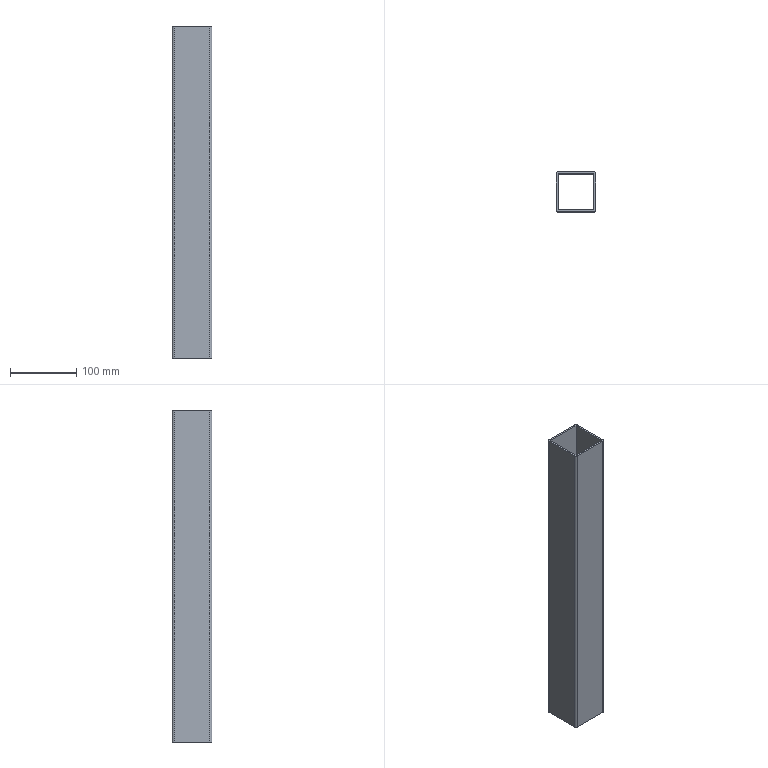Part | STEP file | X77-03111 | 1 solid | 14 faces | box 60 x 60 x 500 mm | volume 338137 mm3 | plane 10 | cylinder 4 | commonest cylinder face diameters 6 x4
STEP:
#1=CARTESIAN_POINT('',(0.,3.,500.));
#2=VERTEX_POINT('',#1);
#3=CARTESIAN_POINT('',(3.,0.,500.));
#4=VERTEX_POINT('',#3);
#5=CARTESIAN_POINT('',(3.,3.,500.));
#6=DIRECTION('',(0.,0.,1.));
#7=DIRECTION('',(1.,0.,0.));
#8=AXIS2_PLACEMENT_3D('',#5,#6,#7);
#9=CIRCLE('',#8,3.);
#10=EDGE_CURVE('',#2,#4,#9,.T.);
#11=ORIENTED_EDGE('',*,*,#10,.T.);
#12=CARTESIAN_POINT('',(57.,0.,500.));
#13=VERTEX_POINT('',#12);
#14=CARTESIAN_POINT('',(3.,0.,500.));
#15=DIRECTION('',(1.,0.,0.));
#16=VECTOR('',#15,1000.);
#17=LINE('',#14,#16);
#18=EDGE_CURVE('',#4,#13,#17,.T.);
#19=ORIENTED_EDGE('',*,*,#18,.T.);
#20=CARTESIAN_POINT('',(60.,3.,500.));
#21=VERTEX_POINT('',#20);
#22=CARTESIAN_POINT('',(57.,3.,500.));
#23=DIRECTION('',(0.,0.,1.));
#24=DIRECTION('',(1.,0.,0.));
#25=AXIS2_PLACEMENT_3D('',#22,#23,#24);
#26=CIRCLE('',#25,3.);
#27=EDGE_CURVE('',#13,#21,#26,.T.);
#28=ORIENTED_EDGE('',*,*,#27,.T.);
#29=CARTESIAN_POINT('',(60.,57.,500.));
#30=VERTEX_POINT('',#29);
#31=CARTESIAN_POINT('',(60.,3.,500.));
#32=DIRECTION('',(0.,1.,0.));
#33=VECTOR('',#32,1000.);
#34=LINE('',#31,#33);
#35=EDGE_CURVE('',#21,#30,#34,.T.);
#36=ORIENTED_EDGE('',*,*,#35,.T.);
#37=CARTESIAN_POINT('',(57.,60.,500.));
#38=VERTEX_POINT('',#37);
#39=CARTESIAN_POINT('',(57.,57.,500.));
#40=DIRECTION('',(0.,0.,1.));
#41=DIRECTION('',(1.,0.,0.));
#42=AXIS2_PLACEMENT_3D('',#39,#40,#41);
#43=CIRCLE('',#42,3.);
#44=EDGE_CURVE('',#30,#38,#43,.T.);
#45=ORIENTED_EDGE('',*,*,#44,.T.);
#46=CARTESIAN_POINT('',(3.,60.,500.));
#47=VERTEX_POINT('',#46);
#48=CARTESIAN_POINT('',(3.,60.,500.));
#49=DIRECTION('',(-1.,0.,0.));
#50=VECTOR('',#49,1000.);
#51=LINE('',#48,#50);
#52=EDGE_CURVE('',#38,#47,#51,.T.);
#53=ORIENTED_EDGE('',*,*,#52,.T.);
#54=CARTESIAN_POINT('',(0.,57.,500.));
#55=VERTEX_POINT('',#54);
#56=CARTESIAN_POINT('',(3.,57.,500.));
#57=DIRECTION('',(0.,0.,1.));
#58=DIRECTION('',(1.,0.,0.));
#59=AXIS2_PLACEMENT_3D('',#56,#57,#58);
#60=CIRCLE('',#59,3.);
#61=EDGE_CURVE('',#47,#55,#60,.T.);
#62=ORIENTED_EDGE('',*,*,#61,.T.);
#63=CARTESIAN_POINT('',(0.,3.,500.));
#64=DIRECTION('',(0.,-1.,0.));
#65=VECTOR('',#64,1000.);
#66=LINE('',#63,#65);
#67=EDGE_CURVE('',#55,#2,#66,.T.);
#68=ORIENTED_EDGE('',*,*,#67,.T.);
#69=EDGE_LOOP('',(#11,#19,#28,#36,#45,#53,#62,#68));
#70=FACE_OUTER_BOUND('',#69,.T.);
#71=CARTESIAN_POINT('',(3.,3.,500.));
#72=VERTEX_POINT('',#71);
#73=CARTESIAN_POINT('',(57.,3.,500.));
#74=VERTEX_POINT('',#73);
#75=CARTESIAN_POINT('',(3.,3.,500.));
#76=DIRECTION('',(1.,0.,0.));
#77=VECTOR('',#76,1000.);
#78=LINE('',#75,#77);
#79=EDGE_CURVE('',#72,#74,#78,.T.);
#80=ORIENTED_EDGE('',*,*,#79,.F.);
#81=CARTESIAN_POINT('',(3.,57.,500.));
#82=VERTEX_POINT('',#81);
#83=CARTESIAN_POINT('',(3.,3.,500.));
#84=DIRECTION('',(0.,-1.,0.));
#85=VECTOR('',#84,1000.);
#86=LINE('',#83,#85);
#87=EDGE_CURVE('',#82,#72,#86,.T.);
#88=ORIENTED_EDGE('',*,*,#87,.F.);
#89=CARTESIAN_POINT('',(57.,57.,500.));
#90=VERTEX_POINT('',#89);
#91=CARTESIAN_POINT('',(3.,57.,500.));
#92=DIRECTION('',(-1.,0.,0.));
#93=VECTOR('',#92,1000.);
#94=LINE('',#91,#93);
#95=EDGE_CURVE('',#90,#82,#94,.T.);
#96=ORIENTED_EDGE('',*,*,#95,.F.);
#97=CARTESIAN_POINT('',(57.,3.,500.));
#98=DIRECTION('',(0.,1.,0.));
#99=VECTOR('',#98,1000.);
#100=LINE('',#97,#99);
#101=EDGE_CURVE('',#74,#90,#100,.T.);
#102=ORIENTED_EDGE('',*,*,#101,.F.);
#103=EDGE_LOOP('',(#80,#88,#96,#102));
#104=FACE_BOUND('',#103,.T.);
#105=CARTESIAN_POINT('',(3.,3.,500.));
#106=DIRECTION('',(0.,0.,1.));
#107=DIRECTION('',(1.,0.,0.));
#108=AXIS2_PLACEMENT_3D('',#105,#106,#107);
#109=PLANE('',#108);
#110=ADVANCED_FACE('',(#70,#104),#109,.T.);
#111=CARTESIAN_POINT('',(0.,3.,0.));
#112=VERTEX_POINT('',#111);
#113=CARTESIAN_POINT('',(3.,0.,0.));
#114=VERTEX_POINT('',#113);
#115=CARTESIAN_POINT('',(3.,3.,0.));
#116=DIRECTION('',(0.,0.,1.));
#117=DIRECTION('',(1.,0.,0.));
#118=AXIS2_PLACEMENT_3D('',#115,#116,#117);
#119=CIRCLE('',#118,3.);
#120=EDGE_CURVE('',#112,#114,#119,.T.);
#121=ORIENTED_EDGE('',*,*,#120,.F.);
#122=CARTESIAN_POINT('',(0.,57.,0.));
#123=VERTEX_POINT('',#122);
#124=CARTESIAN_POINT('',(0.,3.,0.));
#125=DIRECTION('',(0.,-1.,0.));
#126=VECTOR('',#125,1000.);
#127=LINE('',#124,#126);
#128=EDGE_CURVE('',#123,#112,#127,.T.);
#129=ORIENTED_EDGE('',*,*,#128,.F.);
#130=CARTESIAN_POINT('',(3.,60.,0.));
#131=VERTEX_POINT('',#130);
#132=CARTESIAN_POINT('',(3.,57.,0.));
#133=DIRECTION('',(0.,0.,1.));
#134=DIRECTION('',(1.,0.,0.));
#135=AXIS2_PLACEMENT_3D('',#132,#133,#134);
#136=CIRCLE('',#135,3.);
#137=EDGE_CURVE('',#131,#123,#136,.T.);
#138=ORIENTED_EDGE('',*,*,#137,.F.);
#139=CARTESIAN_POINT('',(57.,60.,0.));
#140=VERTEX_POINT('',#139);
#141=CARTESIAN_POINT('',(3.,60.,0.));
#142=DIRECTION('',(-1.,0.,0.));
#143=VECTOR('',#142,1000.);
#144=LINE('',#141,#143);
#145=EDGE_CURVE('',#140,#131,#144,.T.);
#146=ORIENTED_EDGE('',*,*,#145,.F.);
#147=CARTESIAN_POINT('',(60.,57.,0.));
#148=VERTEX_POINT('',#147);
#149=CARTESIAN_POINT('',(57.,57.,0.));
#150=DIRECTION('',(0.,0.,1.));
#151=DIRECTION('',(1.,0.,0.));
#152=AXIS2_PLACEMENT_3D('',#149,#150,#151);
#153=CIRCLE('',#152,3.);
#154=EDGE_CURVE('',#148,#140,#153,.T.);
#155=ORIENTED_EDGE('',*,*,#154,.F.);
#156=CARTESIAN_POINT('',(60.,3.,0.));
#157=VERTEX_POINT('',#156);
#158=CARTESIAN_POINT('',(60.,3.,0.));
#159=DIRECTION('',(0.,1.,0.));
#160=VECTOR('',#159,1000.);
#161=LINE('',#158,#160);
#162=EDGE_CURVE('',#157,#148,#161,.T.);
#163=ORIENTED_EDGE('',*,*,#162,.F.);
#164=CARTESIAN_POINT('',(57.,0.,0.));
#165=VERTEX_POINT('',#164);
#166=CARTESIAN_POINT('',(57.,3.,0.));
#167=DIRECTION('',(0.,0.,1.));
#168=DIRECTION('',(1.,0.,0.));
#169=AXIS2_PLACEMENT_3D('',#166,#167,#168);
#170=CIRCLE('',#169,3.);
#171=EDGE_CURVE('',#165,#157,#170,.T.);
#172=ORIENTED_EDGE('',*,*,#171,.F.);
#173=CARTESIAN_POINT('',(3.,0.,0.));
#174=DIRECTION('',(1.,0.,0.));
#175=VECTOR('',#174,1000.);
#176=LINE('',#173,#175);
#177=EDGE_CURVE('',#114,#165,#176,.T.);
#178=ORIENTED_EDGE('',*,*,#177,.F.);
#179=EDGE_LOOP('',(#121,#129,#138,#146,#155,#163,#172,#178));
#180=FACE_OUTER_BOUND('',#179,.T.);
#181=CARTESIAN_POINT('',(3.,57.,0.));
#182=VERTEX_POINT('',#181);
#183=CARTESIAN_POINT('',(3.,3.,0.));
#184=VERTEX_POINT('',#183);
#185=CARTESIAN_POINT('',(3.,3.,0.));
#186=DIRECTION('',(0.,-1.,0.));
#187=VECTOR('',#186,1000.);
#188=LINE('',#185,#187);
#189=EDGE_CURVE('',#182,#184,#188,.T.);
#190=ORIENTED_EDGE('',*,*,#189,.T.);
#191=CARTESIAN_POINT('',(57.,3.,0.));
#192=VERTEX_POINT('',#191);
#193=CARTESIAN_POINT('',(3.,3.,0.));
#194=DIRECTION('',(1.,0.,0.));
#195=VECTOR('',#194,1000.);
#196=LINE('',#193,#195);
#197=EDGE_CURVE('',#184,#192,#196,.T.);
#198=ORIENTED_EDGE('',*,*,#197,.T.);
#199=CARTESIAN_POINT('',(57.,57.,0.));
#200=VERTEX_POINT('',#199);
#201=CARTESIAN_POINT('',(57.,3.,0.));
#202=DIRECTION('',(0.,1.,0.));
#203=VECTOR('',#202,1000.);
#204=LINE('',#201,#203);
#205=EDGE_CURVE('',#192,#200,#204,.T.);
#206=ORIENTED_EDGE('',*,*,#205,.T.);
#207=CARTESIAN_POINT('',(3.,57.,0.));
#208=DIRECTION('',(-1.,0.,0.));
#209=VECTOR('',#208,1000.);
#210=LINE('',#207,#209);
#211=EDGE_CURVE('',#200,#182,#210,.T.);
#212=ORIENTED_EDGE('',*,*,#211,.T.);
#213=EDGE_LOOP('',(#190,#198,#206,#212));
#214=FACE_BOUND('',#213,.T.);
#215=CARTESIAN_POINT('',(3.,3.,0.));
#216=DIRECTION('',(0.,0.,1.));
#217=DIRECTION('',(1.,0.,0.));
#218=AXIS2_PLACEMENT_3D('',#215,#216,#217);
#219=PLANE('',#218);
#220=ADVANCED_FACE('',(#180,#214),#219,.F.);
#221=ORIENTED_EDGE('',*,*,#120,.T.);
#222=CARTESIAN_POINT('',(3.,0.,500.));
#223=DIRECTION('',(0.,0.,-1.));
#224=VECTOR('',#223,1000.);
#225=LINE('',#222,#224);
#226=EDGE_CURVE('',#4,#114,#225,.T.);
#227=ORIENTED_EDGE('',*,*,#226,.F.);
#228=ORIENTED_EDGE('',*,*,#10,.F.);
#229=CARTESIAN_POINT('',(0.,3.,500.));
#230=DIRECTION('',(0.,0.,-1.));
#231=VECTOR('',#230,1000.);
#232=LINE('',#229,#231);
#233=EDGE_CURVE('',#2,#112,#232,.T.);
#234=ORIENTED_EDGE('',*,*,#233,.T.);
#235=EDGE_LOOP('',(#221,#227,#228,#234));
#236=FACE_OUTER_BOUND('',#235,.T.);
#237=CARTESIAN_POINT('',(3.,3.,500.));
#238=DIRECTION('',(0.,0.,-1.));
#239=DIRECTION('',(-1.,0.,0.));
#240=AXIS2_PLACEMENT_3D('',#237,#238,#239);
#241=CYLINDRICAL_SURFACE('',#240,3.);
#242=ADVANCED_FACE('',(#236),#241,.T.);
#243=ORIENTED_EDGE('',*,*,#177,.T.);
#244=CARTESIAN_POINT('',(57.,0.,500.));
#245=DIRECTION('',(0.,0.,-1.));
#246=VECTOR('',#245,1000.);
#247=LINE('',#244,#246);
#248=EDGE_CURVE('',#13,#165,#247,.T.);
#249=ORIENTED_EDGE('',*,*,#248,.F.);
#250=ORIENTED_EDGE('',*,*,#18,.F.);
#251=ORIENTED_EDGE('',*,*,#226,.T.);
#252=EDGE_LOOP('',(#243,#249,#250,#251));
#253=FACE_OUTER_BOUND('',#252,.T.);
#254=CARTESIAN_POINT('',(3.,0.,500.));
#255=DIRECTION('',(0.,1.,0.));
#256=DIRECTION('',(0.,0.,1.));
#257=AXIS2_PLACEMENT_3D('',#254,#255,#256);
#258=PLANE('',#257);
#259=ADVANCED_FACE('',(#253),#258,.F.);
#260=ORIENTED_EDGE('',*,*,#171,.T.);
#261=CARTESIAN_POINT('',(60.,3.,500.));
#262=DIRECTION('',(0.,0.,-1.));
#263=VECTOR('',#262,1000.);
#264=LINE('',#261,#263);
#265=EDGE_CURVE('',#21,#157,#264,.T.);
#266=ORIENTED_EDGE('',*,*,#265,.F.);
#267=ORIENTED_EDGE('',*,*,#27,.F.);
#268=ORIENTED_EDGE('',*,*,#248,.T.);
#269=EDGE_LOOP('',(#260,#266,#267,#268));
#270=FACE_OUTER_BOUND('',#269,.T.);
#271=CARTESIAN_POINT('',(57.,3.,500.));
#272=DIRECTION('',(0.,0.,-1.));
#273=DIRECTION('',(-1.,0.,0.));
#274=AXIS2_PLACEMENT_3D('',#271,#272,#273);
#275=CYLINDRICAL_SURFACE('',#274,3.);
#276=ADVANCED_FACE('',(#270),#275,.T.);
#277=ORIENTED_EDGE('',*,*,#162,.T.);
#278=CARTESIAN_POINT('',(60.,57.,500.));
#279=DIRECTION('',(0.,0.,-1.));
#280=VECTOR('',#279,1000.);
#281=LINE('',#278,#280);
#282=EDGE_CURVE('',#30,#148,#281,.T.);
#283=ORIENTED_EDGE('',*,*,#282,.F.);
#284=ORIENTED_EDGE('',*,*,#35,.F.);
#285=ORIENTED_EDGE('',*,*,#265,.T.);
#286=EDGE_LOOP('',(#277,#283,#284,#285));
#287=FACE_OUTER_BOUND('',#286,.T.);
#288=CARTESIAN_POINT('',(60.,3.,500.));
#289=DIRECTION('',(-1.,0.,0.));
#290=DIRECTION('',(0.,0.,1.));
#291=AXIS2_PLACEMENT_3D('',#288,#289,#290);
#292=PLANE('',#291);
#293=ADVANCED_FACE('',(#287),#292,.F.);
#294=ORIENTED_EDGE('',*,*,#154,.T.);
#295=CARTESIAN_POINT('',(57.,60.,500.));
#296=DIRECTION('',(0.,0.,-1.));
#297=VECTOR('',#296,1000.);
#298=LINE('',#295,#297);
#299=EDGE_CURVE('',#38,#140,#298,.T.);
#300=ORIENTED_EDGE('',*,*,#299,.F.);
#301=ORIENTED_EDGE('',*,*,#44,.F.);
#302=ORIENTED_EDGE('',*,*,#282,.T.);
#303=EDGE_LOOP('',(#294,#300,#301,#302));
#304=FACE_OUTER_BOUND('',#303,.T.);
#305=CARTESIAN_POINT('',(57.,57.,500.));
#306=DIRECTION('',(0.,0.,-1.));
#307=DIRECTION('',(-1.,0.,0.));
#308=AXIS2_PLACEMENT_3D('',#305,#306,#307);
#309=CYLINDRICAL_SURFACE('',#308,3.);
#310=ADVANCED_FACE('',(#304),#309,.T.);
#311=ORIENTED_EDGE('',*,*,#145,.T.);
#312=CARTESIAN_POINT('',(3.,60.,500.));
#313=DIRECTION('',(0.,0.,-1.));
#314=VECTOR('',#313,1000.);
#315=LINE('',#312,#314);
#316=EDGE_CURVE('',#47,#131,#315,.T.);
#317=ORIENTED_EDGE('',*,*,#316,.F.);
#318=ORIENTED_EDGE('',*,*,#52,.F.);
#319=ORIENTED_EDGE('',*,*,#299,.T.);
#320=EDGE_LOOP('',(#311,#317,#318,#319));
#321=FACE_OUTER_BOUND('',#320,.T.);
#322=CARTESIAN_POINT('',(3.,60.,500.));
#323=DIRECTION('',(0.,-1.,0.));
#324=DIRECTION('',(0.,0.,-1.));
#325=AXIS2_PLACEMENT_3D('',#322,#323,#324);
#326=PLANE('',#325);
#327=ADVANCED_FACE('',(#321),#326,.F.);
#328=ORIENTED_EDGE('',*,*,#137,.T.);
#329=CARTESIAN_POINT('',(0.,57.,500.));
#330=DIRECTION('',(0.,0.,-1.));
#331=VECTOR('',#330,1000.);
#332=LINE('',#329,#331);
#333=EDGE_CURVE('',#55,#123,#332,.T.);
#334=ORIENTED_EDGE('',*,*,#333,.F.);
#335=ORIENTED_EDGE('',*,*,#61,.F.);
#336=ORIENTED_EDGE('',*,*,#316,.T.);
#337=EDGE_LOOP('',(#328,#334,#335,#336));
#338=FACE_OUTER_BOUND('',#337,.T.);
#339=CARTESIAN_POINT('',(3.,57.,500.));
#340=DIRECTION('',(0.,0.,-1.));
#341=DIRECTION('',(-1.,0.,0.));
#342=AXIS2_PLACEMENT_3D('',#339,#340,#341);
#343=CYLINDRICAL_SURFACE('',#342,3.);
#344=ADVANCED_FACE('',(#338),#343,.T.);
#345=ORIENTED_EDGE('',*,*,#128,.T.);
#346=ORIENTED_EDGE('',*,*,#233,.F.);
#347=ORIENTED_EDGE('',*,*,#67,.F.);
#348=ORIENTED_EDGE('',*,*,#333,.T.);
#349=EDGE_LOOP('',(#345,#346,#347,#348));
#350=FACE_OUTER_BOUND('',#349,.T.);
#351=CARTESIAN_POINT('',(0.,3.,500.));
#352=DIRECTION('',(1.,0.,0.));
#353=DIRECTION('',(0.,0.,-1.));
#354=AXIS2_PLACEMENT_3D('',#351,#352,#353);
#355=PLANE('',#354);
#356=ADVANCED_FACE('',(#350),#355,.F.);
#357=ORIENTED_EDGE('',*,*,#189,.F.);
#358=CARTESIAN_POINT('',(3.,57.,500.));
#359=DIRECTION('',(0.,0.,-1.));
#360=VECTOR('',#359,1000.);
#361=LINE('',#358,#360);
#362=EDGE_CURVE('',#82,#182,#361,.T.);
#363=ORIENTED_EDGE('',*,*,#362,.F.);
#364=ORIENTED_EDGE('',*,*,#87,.T.);
#365=CARTESIAN_POINT('',(3.,3.,500.));
#366=DIRECTION('',(0.,0.,-1.));
#367=VECTOR('',#366,1000.);
#368=LINE('',#365,#367);
#369=EDGE_CURVE('',#72,#184,#368,.T.);
#370=ORIENTED_EDGE('',*,*,#369,.T.);
#371=EDGE_LOOP('',(#357,#363,#364,#370));
#372=FACE_OUTER_BOUND('',#371,.T.);
#373=CARTESIAN_POINT('',(3.,3.,500.));
#374=DIRECTION('',(1.,0.,0.));
#375=DIRECTION('',(0.,0.,-1.));
#376=AXIS2_PLACEMENT_3D('',#373,#374,#375);
#377=PLANE('',#376);
#378=ADVANCED_FACE('',(#372),#377,.T.);
#379=ORIENTED_EDGE('',*,*,#197,.F.);
#380=ORIENTED_EDGE('',*,*,#369,.F.);
#381=ORIENTED_EDGE('',*,*,#79,.T.);
#382=CARTESIAN_POINT('',(57.,3.,500.));
#383=DIRECTION('',(0.,0.,-1.));
#384=VECTOR('',#383,1000.);
#385=LINE('',#382,#384);
#386=EDGE_CURVE('',#74,#192,#385,.T.);
#387=ORIENTED_EDGE('',*,*,#386,.T.);
#388=EDGE_LOOP('',(#379,#380,#381,#387));
#389=FACE_OUTER_BOUND('',#388,.T.);
#390=CARTESIAN_POINT('',(3.,3.,500.));
#391=DIRECTION('',(0.,1.,0.));
#392=DIRECTION('',(0.,0.,1.));
#393=AXIS2_PLACEMENT_3D('',#390,#391,#392);
#394=PLANE('',#393);
#395=ADVANCED_FACE('',(#389),#394,.T.);
#396=ORIENTED_EDGE('',*,*,#205,.F.);
#397=ORIENTED_EDGE('',*,*,#386,.F.);
#398=ORIENTED_EDGE('',*,*,#101,.T.);
#399=CARTESIAN_POINT('',(57.,57.,500.));
#400=DIRECTION('',(0.,0.,-1.));
#401=VECTOR('',#400,1000.);
#402=LINE('',#399,#401);
#403=EDGE_CURVE('',#90,#200,#402,.T.);
#404=ORIENTED_EDGE('',*,*,#403,.T.);
#405=EDGE_LOOP('',(#396,#397,#398,#404));
#406=FACE_OUTER_BOUND('',#405,.T.);
#407=CARTESIAN_POINT('',(57.,3.,500.));
#408=DIRECTION('',(-1.,0.,0.));
#409=DIRECTION('',(0.,0.,1.));
#410=AXIS2_PLACEMENT_3D('',#407,#408,#409);
#411=PLANE('',#410);
#412=ADVANCED_FACE('',(#406),#411,.T.);
#413=ORIENTED_EDGE('',*,*,#211,.F.);
#414=ORIENTED_EDGE('',*,*,#403,.F.);
#415=ORIENTED_EDGE('',*,*,#95,.T.);
#416=ORIENTED_EDGE('',*,*,#362,.T.);
#417=EDGE_LOOP('',(#413,#414,#415,#416));
#418=FACE_OUTER_BOUND('',#417,.T.);
#419=CARTESIAN_POINT('',(3.,57.,500.));
#420=DIRECTION('',(0.,-1.,0.));
#421=DIRECTION('',(0.,0.,-1.));
#422=AXIS2_PLACEMENT_3D('',#419,#420,#421);
#423=PLANE('',#422);
#424=ADVANCED_FACE('',(#418),#423,.T.);
#425=CLOSED_SHELL('',(#110,#220,#242,#259,#276,#293,#310,#327,#344,#356,#378,#395,#412,#424));
#426=MANIFOLD_SOLID_BREP('',#425);
#427=CARTESIAN_POINT('',(0.,0.,0.));
#428=DIRECTION('',(0.,0.,1.));
#429=DIRECTION('',(1.,0.,0.));
#430=AXIS2_PLACEMENT_3D('',#427,#428,#429);
#431=(LENGTH_UNIT()NAMED_UNIT(*)SI_UNIT(.MILLI.,.METRE.));
#432=UNCERTAINTY_MEASURE_WITH_UNIT(LENGTH_MEASURE(0.00001),#431,'','');
#433=(NAMED_UNIT(*)PLANE_ANGLE_UNIT()SI_UNIT($,.RADIAN.));
#434=(NAMED_UNIT(*)SI_UNIT($,.STERADIAN.)SOLID_ANGLE_UNIT());
#435=(GEOMETRIC_REPRESENTATION_CONTEXT(3)GLOBAL_UNCERTAINTY_ASSIGNED_CONTEXT((#432))GLOBAL_UNIT_ASSIGNED_CONTEXT((#431,#433,#434))REPRESENTATION_CONTEXT('',''));
#436=ADVANCED_BREP_SHAPE_REPRESENTATION('',(#426,#430),#435);